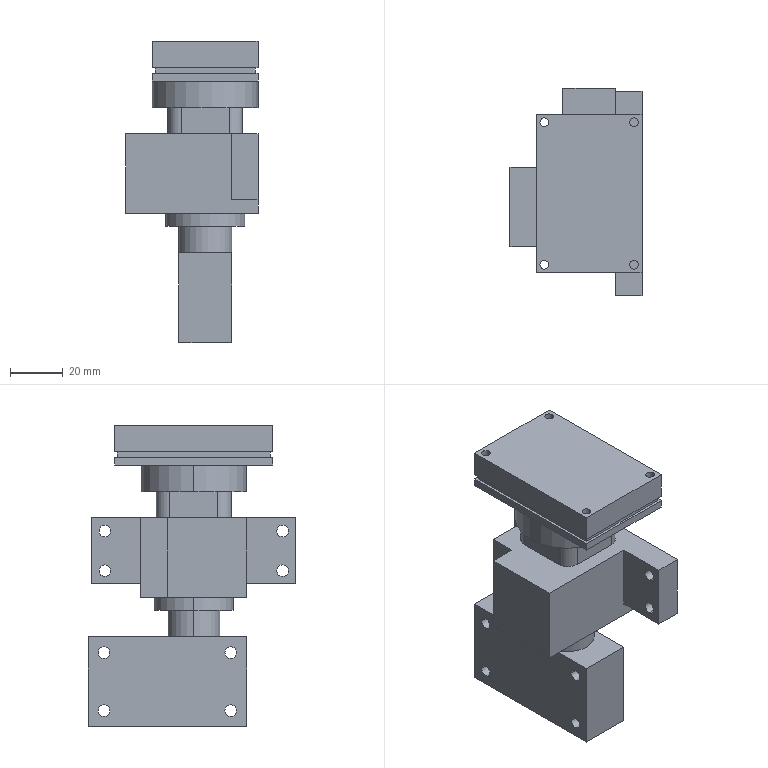Part | SolidWorks | features MirrorStock 1 | 1 solid | 78 faces | box 50 x 78.682 x 114 mm | volume 167439 mm3 | plane 44 | cylinder 34 | commonest cylinder face diameters 4.4 x16 3.3 x8 10 x4 20 x2 30 x2 40 x2